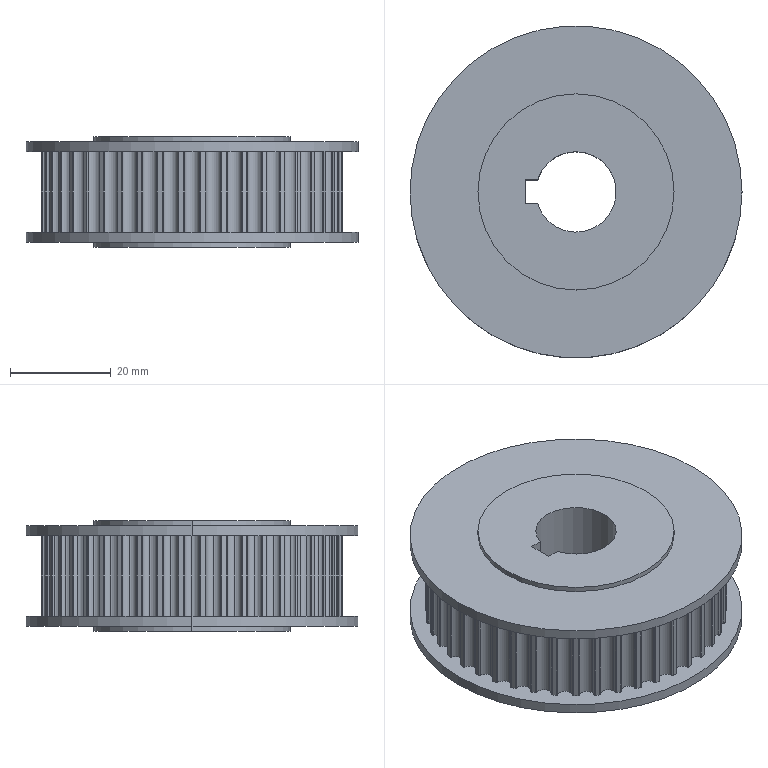Part | SolidWorks | features ICE 6, CirPattern 1, Extrusion 1, Fillet 1 | 1 solid | 233 faces | box 66 x 66 x 22 mm | volume 54187 mm3 | cylinder 224 | plane 9 | commonest cylinder face diameters 0.4 x108 3 x63 60 x44 39 x4 66 x4 16 x1